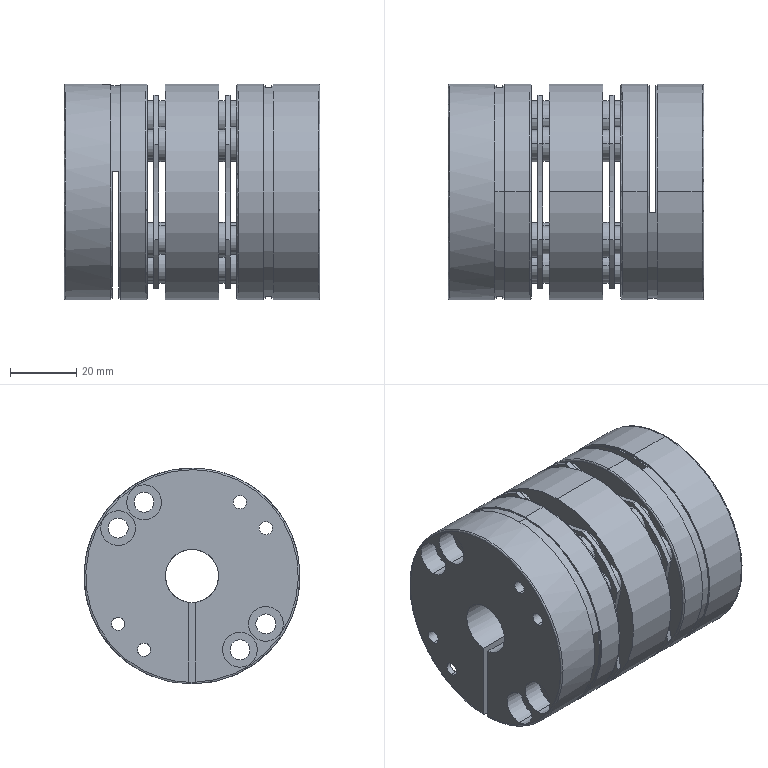Part | STEP file | 0244_Z_007_CPSWC65-16-20_1 | 1 solid | 221 faces | box 77 x 65 x 65 mm | volume 173127 mm3 | cylinder 172 | plane 40 | spline 9 | commonest cylinder face diameters 10.5 x48 8.5 x32 4 x20 65 x18 6 x16 100 x10